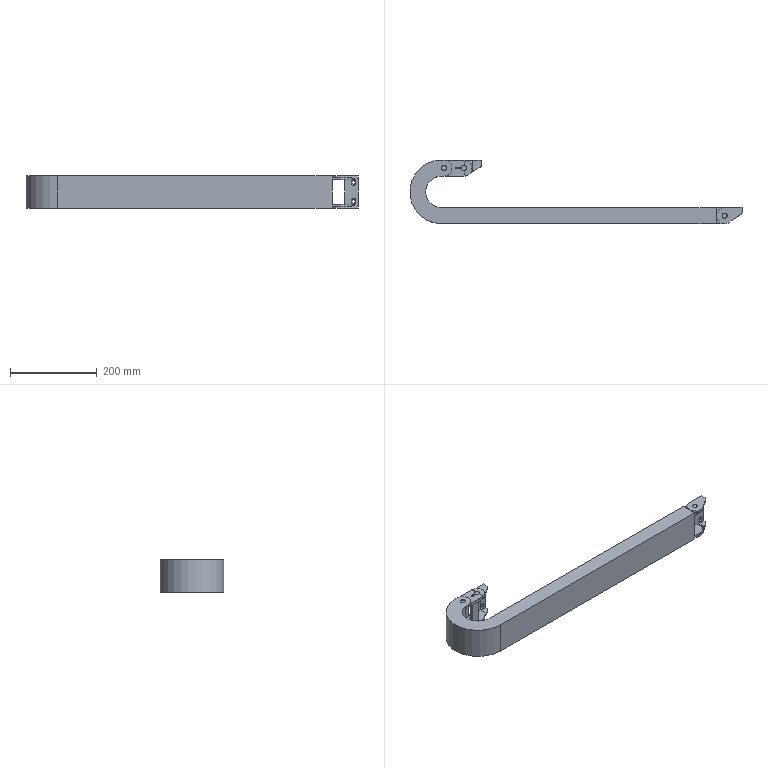Part | SolidWorks | features BaseBody 4 | 4 solids | 358 faces | box 767.5 x 147.5 x 74 mm | volume 1154878 mm3 | plane 247 | cylinder 99 | cone 12 | commonest cylinder face diameters 37 x23 2 x12 4 x12 6.6 x12 12 x12 12.1 x8